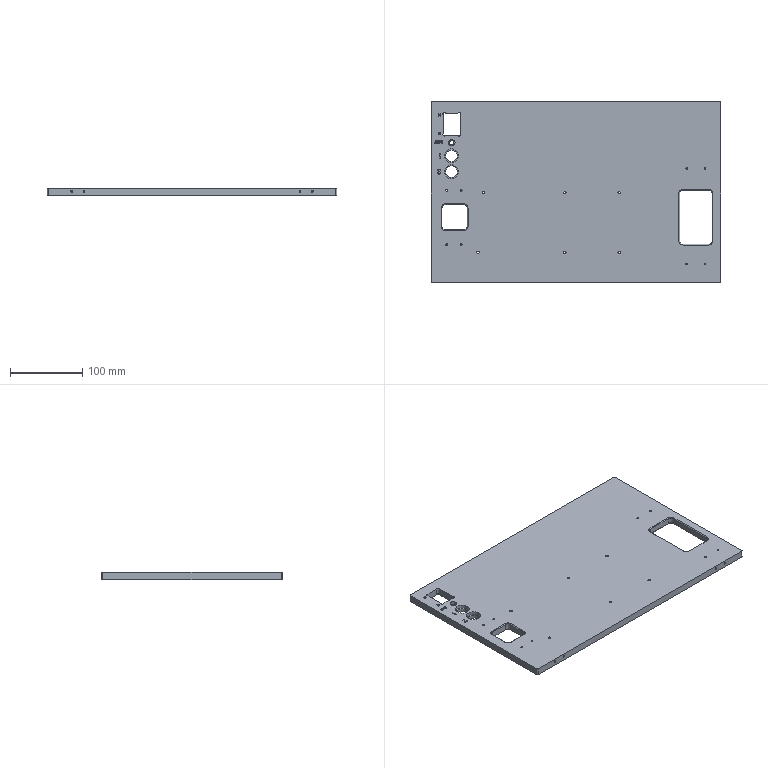Part | 1 solid | 345 faces | box 400 x 250 x 10 mm | volume 940317 mm3 | plane 187 | cylinder 70 | spline 64 | cone 24 | commonest cylinder face diameters 2.5 x28 3.3 x12 10 x8 4.2 x6 3 x4 16 x4